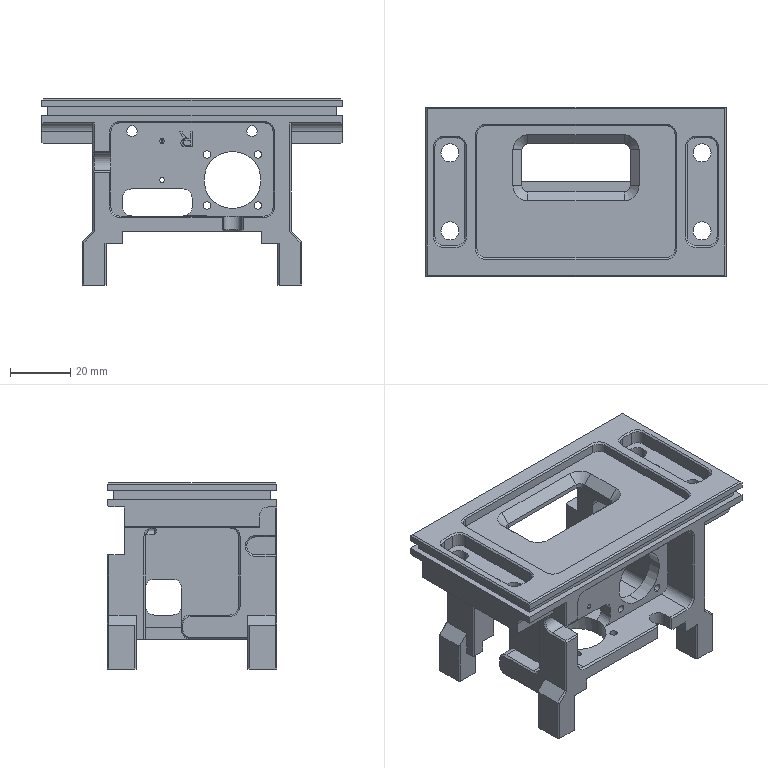NC program | Mastercam | posted with a generic post | part box 100 x 56.5 x 62 mm
Lines 34 to 1359 of 47040:
N260 T13 M6
N270 G0 G90 G17 G54 X-64.057 Y-49.411 A0. S5500 M3
N280 G43 H13 Z20. M8
N290 Z1.
N300 G1 Z-28.25 F600.
N310 X-64.59 Y-48.087 Z-28.374 F3000.
N320 G3 X-65.384 Y-46.884 Z-28.5 I-3.34 J-1.343
N330 G1 X-65.592 Y-46.603
N340 X-66.057 Y-45.951
N350 X-66.342 Y-45.52
N360 X-66.635 Y-45.037
N370 X-66.924 Y-44.51
N380 X-67.198 Y-43.943
N390 X-67.451 Y-43.341
N400 X-67.673 Y-42.718
N410 X-67.849 Y-42.127
N420 X-67.986 Y-41.577
N430 X-68.092 Y-41.064
N440 X-68.174 Y-40.586
N450 X-68.238 Y-40.138
N460 X-68.326 Y-39.34
N470 X-68.382 Y-38.609
N480 X-68.418 Y-37.931
N490 X-68.441 Y-37.291
N500 X-68.456 Y-36.678
N510 X-68.465 Y-36.084
N520 X-68.471 Y-35.505
N530 X-68.474 Y-34.935
N540 X-68.475 Y-34.371
N550 X-68.476 Y-33.813
N560 X-68.475 Y-33.258
N570 X-68.474 Y-32.705
N580 X-68.473 Y-32.153
N590 X-68.472 Y-31.603
N600 X-68.471 Y-31.052
N610 X-68.469 Y-30.502
N620 X-68.467 Y-29.953
N630 X-68.466 Y-29.403
N640 X-68.464 Y-28.853
N650 X-68.463 Y-28.304
N660 X-68.461 Y-27.754
N670 X-68.459 Y-27.205
N680 X-68.458 Y-26.655
N690 X-68.456 Y-26.105
N700 X-68.455 Y-25.556
N710 X-68.453 Y-25.006
N720 X-68.451 Y-24.456
N730 X-68.45 Y-23.906
N740 X-68.448 Y-23.357
N750 X-68.446 Y-22.807
N760 X-68.445 Y-22.257
N770 X-68.443 Y-21.707
N780 X-68.442 Y-21.157
N790 X-68.44 Y-20.607
N800 X-68.438 Y-20.057
N810 X-68.437 Y-19.507
N820 X-68.435 Y-18.957
N830 X-68.433 Y-18.407
N840 X-68.432 Y-17.857
N850 X-68.43 Y-17.307
N860 X-68.429 Y-16.757
N870 X-68.427 Y-16.207
N880 X-68.425 Y-15.656
N890 X-68.424 Y-15.106
N900 X-68.422 Y-14.556
N910 X-68.42 Y-14.006
N920 X-68.419 Y-13.456
N930 X-68.417 Y-12.905
N940 X-68.416 Y-12.355
N950 X-68.414 Y-11.805
N960 X-68.412 Y-11.254
N970 X-68.411 Y-10.704
N980 X-68.409 Y-10.153
N990 X-68.407 Y-9.603
N1000 X-68.406 Y-9.052
N1010 X-68.404 Y-8.502
N1020 X-68.403 Y-7.951
N1030 X-68.401 Y-7.401
N1040 X-68.399 Y-6.85
N1050 X-68.398 Y-6.3
N1060 X-68.396 Y-5.749
N1070 X-68.394 Y-5.199
N1080 X-68.393 Y-4.648
N1090 X-68.391 Y-4.097
N1100 X-68.39 Y-3.547
N1110 X-68.388 Y-2.996
N1120 X-68.386 Y-2.445
N1130 X-68.385 Y-1.895
N1140 X-68.383 Y-1.344
N1150 X-68.381 Y-.793
N1160 X-68.38 Y-.242
N1170 X-68.378 Y.309
N1180 X-68.377 Y.859
N1190 X-68.375 Y1.41
N1200 X-68.373 Y1.961
N1210 X-68.372 Y2.512
N1220 X-68.37 Y3.063
N1230 X-68.368 Y3.614
N1240 X-68.367 Y4.165
N1250 X-68.365 Y4.716
N1260 X-68.363 Y5.267
N1270 X-68.362 Y5.818
N1280 X-68.36 Y6.369
N1290 X-68.359 Y6.92
N1300 X-68.357 Y7.471
N1310 X-68.355 Y8.022
N1320 X-68.354 Y8.573
N1330 X-68.352 Y9.124
N1340 X-68.35 Y9.675
N1350 X-68.349 Y10.226
N1360 X-68.347 Y10.778
N1370 X-68.346 Y11.329
N1380 X-68.344 Y11.88
N1390 X-68.342 Y12.431
N1400 X-68.341 Y12.982
N1410 X-68.339 Y13.534
N1420 X-68.337 Y14.085
N1430 X-68.336 Y14.636
N1440 X-68.334 Y15.187
N1450 X-68.333 Y15.739
N1460 X-68.331 Y16.29
N1470 X-68.329 Y16.841
N1480 X-68.328 Y17.393
N1490 X-68.326 Y17.944
N1500 X-68.324 Y18.495
N1510 X-68.323 Y19.047
N1520 X-68.321 Y19.598
N1530 X-68.319 Y20.149
N1540 X-68.318 Y20.701
N1550 X-68.316 Y21.252
N1560 X-68.315 Y21.804
N1570 X-68.313 Y22.355
N1580 X-68.311 Y22.907
N1590 X-68.31 Y23.458
N1600 X-68.308 Y24.01
N1610 X-68.306 Y24.561
N1620 X-68.305 Y25.113
N1630 X-68.303 Y25.664
N1640 X-68.302 Y26.216
N1650 X-68.3 Y26.767
N1660 X-68.298 Y27.319
N1670 X-68.297 Y27.871
N1680 X-68.295 Y28.422
N1690 X-68.293 Y28.974
N1700 X-68.292 Y29.525
N1710 X-68.29 Y30.077
N1720 X-68.288 Y30.629
N1730 X-68.287 Y31.18
N1740 X-68.285 Y31.732
N1750 X-68.284 Y32.284
N1760 X-68.282 Y32.836
N1770 X-68.28 Y33.387
N1780 X-68.279 Y33.939
N1790 X-68.277 Y34.491
N1800 X-68.275 Y35.043
N1810 X-68.274 Y35.594
N1820 X-68.272 Y36.146
N1830 X-68.27 Y36.705
N1840 X-68.26 Y37.428
N1850 X-68.241 Y37.868
N1860 X-68.208 Y38.345
N1870 X-68.157 Y38.854
N1880 X-68.082 Y39.387
N1890 X-67.981 Y39.94
N1900 X-67.852 Y40.507
N1910 X-67.69 Y41.084
N1920 X-67.495 Y41.665
N1930 X-67.265 Y42.248
N1940 X-66.998 Y42.826
N1950 X-66.694 Y43.397
N1960 X-66.352 Y43.955
N1970 X-65.973 Y44.498
N1980 X-65.558 Y45.022
N1990 X-65.107 Y45.522
N2000 X-64.621 Y45.996
N2010 X-64.106 Y46.436
N2020 X-63.582 Y46.831
N2030 X-63.056 Y47.181
N2040 X-62.533 Y47.489
N2050 X-62.016 Y47.76
N2060 X-61.509 Y47.998
N2070 X-61.014 Y48.205
N2080 X-60.531 Y48.386
N2090 X-60.061 Y48.543
N2100 X-59.605 Y48.681
N2110 X-59.163 Y48.8
N2120 X-58.733 Y48.904
N2130 X-57.927 Y49.071
N2140 X-57.16 Y49.201
N2150 X-56.428 Y49.301
N2160 X-55.726 Y49.378
N2170 X-55.05 Y49.439
N2180 X-54.397 Y49.486
N2190 X-53.761 Y49.523
N2200 X-53.141 Y49.552
N2210 X-52.533 Y49.574
N2220 X-51.936 Y49.592
N2230 X-51.347 Y49.606
N2240 X-50.765 Y49.616
N2250 X-50.189 Y49.624
N2260 X-49.617 Y49.63
N2270 X-49.049 Y49.635
N2280 X-48.485 Y49.638
N2290 X-47.923 Y49.64
N2300 X-47.361 Y49.642
N2310 X-46.801 Y49.643
N2320 X-46.241 Y49.645
N2330 X-45.681 Y49.646
N2340 X-45.123
N2350 X-44.564 Y49.647
N2360 X-44.006 Y49.648
N2370 X-43.448
N2380 X-42.89
N2390 X-42.332 Y49.649
N2400 X-41.775
N2410 X-41.218
N2420 X-40.66
N2430 X-40.103
N2440 X-39.546
N2450 X-38.989 Y49.65
N2460 X-38.432
N2470 X-37.874
N2480 X-37.317
N2490 X-36.76
N2500 X-36.203
N2510 X-35.646
N2520 X-35.089
N2530 X-34.532
N2540 X-33.976
N2550 X-33.419
N2560 X-32.862
N2570 X-32.305
N2580 X-31.748
N2590 X-31.191
N2600 X-30.634
N2610 X-30.077
N2620 X-29.52
N2630 X-28.963
N2640 X-28.406
N2650 X-27.849
N2660 X-27.292
N2670 X-26.735
N2680 X-26.179
N2690 X-25.622
N2700 X-25.065
N2710 X-24.508
N2720 X-23.951
N2730 X-23.394
N2740 X-22.837
N2750 X-22.28
N2760 X-21.723
N2770 X-21.166
N2780 X-20.609
N2790 X-20.053
N2800 X-19.496
N2810 X-18.939
N2820 X-18.382
N2830 X-17.825
N2840 X-17.268
N2850 X-16.711
N2860 X-16.154
N2870 X-15.597
N2880 X-15.04
N2890 X-14.483
N2900 X-13.927
N2910 X-13.37
N2920 X-12.813
N2930 X-12.256
N2940 X-11.699
N2950 X-11.142
N2960 X-10.585
N2970 X-10.028
N2980 X-9.471
N2990 X-8.914
N3000 X-8.357
N3010 X-7.801
N3020 X-7.244
N3030 X-6.687
N3040 X-6.13
N3050 X-5.573
N3060 X-5.016
N3070 X-4.459
N3080 X-3.902
N3090 X-3.345
N3100 X-2.788
N3110 X-2.231
N3120 X-1.675
N3130 X-1.118
N3140 X-.561
N3150 X-.004
N3160 X.553
N3170 X1.11
N3180 X1.667
N3190 X2.224
N3200 X2.781
N3210 X3.338
N3220 X3.895
N3230 X4.452
N3240 X5.008
N3250 X5.565
N3260 X6.122
N3270 X6.679
N3280 X7.236
N3290 X7.793
N3300 X8.35
N3310 X8.907
N3320 X9.464
N3330 X10.021
N3340 X10.578
N3350 X11.134
N3360 X11.691
N3370 X12.248
N3380 X12.805
N3390 X13.362
N3400 X13.919
N3410 X14.476
N3420 X15.033
N3430 X15.59
N3440 X16.147
N3450 X16.704
N3460 X17.26
N3470 X17.817
N3480 X18.374
N3490 X18.931
N3500 X19.488
N3510 X20.045
N3520 X20.602
N3530 X21.159
N3540 X21.716
N3550 X22.273
N3560 X22.83
N3570 X23.386
N3580 X23.943
N3590 X24.5
N3600 X25.057
N3610 X25.614
N3620 X26.171
N3630 X26.728
N3640 X27.285
N3650 X27.842
N3660 X28.399
N3670 X28.956
N3680 X29.512
N3690 X30.069
N3700 X30.626
N3710 X31.183
N3720 X31.74
N3730 X32.297
N3740 X32.854
N3750 X33.411
N3760 X33.968
N3770 X34.525
N3780 X35.082
N3790 X35.638
N3800 X36.195
N3810 X36.752
N3820 X37.309
N3830 X37.866
N3840 X38.423
N3850 X38.98
N3860 X39.537
N3870 X40.094
N3880 X40.651
N3890 X41.208
N3900 X41.765
N3910 X42.321
N3920 X42.878
N3930 X43.435
N3940 X43.992
N3950 X44.549
N3960 X45.106
N3970 X45.663
N3980 X46.22
N3990 X46.777
N4000 X47.334
N4010 X47.891
N4020 X48.447
N4030 X49.004
N4040 X49.561
N4050 X50.118
N4060 X50.675
N4070 X51.232
N4080 X51.789
N4090 X52.346
N4100 X52.903
N4110 X53.46
N4120 X54.017
N4130 X54.573
N4140 X55.19 Y49.649
N4150 X55.986 Y49.629
N4160 X56.447 Y49.602
N4170 X56.938 Y49.559
N4180 X57.453 Y49.495
N4190 X57.988 Y49.409
N4200 X58.538 Y49.296
N4210 X59.1 Y49.154
N4220 X59.667 Y48.981
N4230 X60.238 Y48.776
N4240 X60.807 Y48.536
N4250 X61.372 Y48.26
N4260 X61.927 Y47.949
N4270 X62.47 Y47.602
N4280 X62.996 Y47.218
N4290 X63.503 Y46.8
N4300 X63.986 Y46.346
N4310 X64.439 Y45.864
N4320 X64.85 Y45.368
N4330 X65.221 Y44.865
N4340 X65.553 Y44.36
N4350 X65.85 Y43.856
N4360 X66.113 Y43.356
N4370 X66.347 Y42.864
N4380 X66.554 Y42.38
N4390 X66.737 Y41.907
N4400 X66.898 Y41.444
N4410 X67.04 Y40.992
N4420 X67.165 Y40.552
N4430 X67.276 Y40.123
N4440 X67.456 Y39.314
N4450 X67.597 Y38.541
N4460 X67.708 Y37.8
N4470 X67.796 Y37.089
N4480 X67.866 Y36.403
N4490 X67.921 Y35.738
N4500 X67.965 Y35.092
N4510 X68. Y34.461
N4520 X68.029 Y33.843
N4530 X68.052 Y33.236
N4540 X68.07 Y32.638
N4550 X68.085 Y32.047
N4560 X68.097 Y31.462
N4570 X68.107 Y30.882
N4580 X68.115 Y30.306
N4590 X68.121 Y29.734
N4600 X68.127 Y29.164
N4610 X68.131 Y28.597
N4620 X68.134 Y28.031
N4630 X68.137 Y27.467
N4640 X68.14 Y26.905
N4650 X68.141 Y26.343
N4660 X68.143 Y25.783
N4670 X68.144 Y25.223
N4680 X68.145 Y24.663
N4690 X68.146 Y24.104
N4700 X68.147 Y23.545
N4710 Y22.987
N4720 X68.148 Y22.429
N4730 Y21.871
N4740 X68.149 Y21.314
N4750 Y20.756
N4760 Y20.199
N4770 Y19.641
N4780 Y19.084
N4790 Y18.527
N4800 X68.15 Y17.97
N4810 Y17.413
N4820 Y16.855
N4830 Y16.298
N4840 Y15.741
N4850 Y15.184
N4860 Y14.627
N4870 Y14.07
N4880 Y13.513
N4890 Y12.956
N4900 Y12.4
N4910 Y11.843
N4920 Y11.286
N4930 Y10.729
N4940 Y10.172
N4950 Y9.615
N4960 Y9.058
N4970 Y8.501
N4980 Y7.944
N4990 Y7.387
N5000 Y6.83
N5010 Y6.273
N5020 Y5.716
N5030 Y5.16
N5040 Y4.603
N5050 Y4.046
N5060 Y3.489
N5070 Y2.932
N5080 Y2.375
N5090 Y1.818
N5100 Y1.261
N5110 Y.704
N5120 Y.147
N5130 Y-.41
N5140 Y-.967
N5150 Y-1.523
N5160 Y-2.08
N5170 Y-2.637
N5180 Y-3.194
N5190 Y-3.751
N5200 Y-4.308
N5210 Y-4.865
N5220 Y-5.422
N5230 Y-5.979
N5240 Y-6.536
N5250 Y-7.093
N5260 Y-7.649
N5270 Y-8.206
N5280 Y-8.763
N5290 Y-9.32
N5300 Y-9.877
N5310 Y-10.434
N5320 Y-10.991
N5330 Y-11.548
N5340 Y-12.105
N5350 Y-12.662
N5360 Y-13.219
N5370 Y-13.775
N5380 Y-14.332
N5390 Y-14.889
N5400 Y-15.446
N5410 Y-16.003
N5420 Y-16.56
N5430 Y-17.117
N5440 Y-17.674
N5450 Y-18.231
N5460 Y-18.788
N5470 Y-19.345
N5480 Y-19.901
N5490 Y-20.458
N5500 Y-21.015
N5510 Y-21.572
N5520 Y-22.129
N5530 Y-22.686
N5540 Y-23.243
N5550 Y-23.8
N5560 Y-24.357
N5570 Y-24.914
N5580 Y-25.471
N5590 Y-26.027
N5600 Y-26.584
N5610 Y-27.141
N5620 Y-27.698
N5630 Y-28.255
N5640 Y-28.812
N5650 Y-29.369
N5660 Y-29.926
N5670 Y-30.483
N5680 Y-31.04
N5690 Y-31.597
N5700 Y-32.153
N5710 Y-32.71
N5720 Y-33.267
N5730 Y-33.824
N5740 Y-34.381
N5750 Y-34.938
N5760 Y-35.495
N5770 Y-36.052
N5780 X68.149 Y-36.662
N5790 X68.13 Y-37.452
N5800 X68.104 Y-37.911
N5810 X68.062 Y-38.399
N5820 X68.001 Y-38.913
N5830 X67.916 Y-39.447
N5840 X67.805 Y-39.996
N5850 X67.666 Y-40.557
N5860 X67.496 Y-41.124
N5870 X67.292 Y-41.695
N5880 X67.055 Y-42.264
N5890 X66.782 Y-42.829
N5900 X66.474 Y-43.385
N5910 X66.129 Y-43.929
N5920 X65.749 Y-44.457
N5930 X65.333 Y-44.965
N5940 X64.882 Y-45.45
N5950 X64.401 Y-45.906
N5960 X63.906 Y-46.32
N5970 X63.403 Y-46.694
N5980 X62.898 Y-47.029
N5990 X62.394 Y-47.328
N6000 X61.894 Y-47.595
N6010 X61.401 Y-47.831
N6020 X60.917 Y-48.039
N6030 X60.442 Y-48.224
N6040 X59.979 Y-48.386
N6050 X59.526 Y-48.53
N6060 X59.085 Y-48.656
N6070 X58.655 Y-48.768
N6080 X57.844 Y-48.95
N6090 X57.07 Y-49.092
N6100 X56.328 Y-49.205
N6110 X55.616 Y-49.293
N6120 X54.929 Y-49.363
N6130 X54.264 Y-49.419
N6140 X53.617 Y-49.464
N6150 X52.985 Y-49.499
N6160 X52.367 Y-49.528
N6170 X51.759 Y-49.551
N6180 X51.161 Y-49.569
N6190 X50.569 Y-49.584
N6200 X49.984 Y-49.597
N6210 X49.404 Y-49.606
N6220 X48.828 Y-49.614
N6230 X48.256 Y-49.621
N6240 X47.686 Y-49.626
N6250 X47.119 Y-49.631
N6260 X46.553 Y-49.634
N6270 X45.989 Y-49.637
N6280 X45.427 Y-49.639
N6290 X44.865 Y-49.641
N6300 X44.304 Y-49.643
N6310 X43.744 Y-49.644
N6320 X43.185 Y-49.645
N6330 X42.626 Y-49.646
N6340 X42.067 Y-49.647
N6350 X41.509
N6360 X40.951 Y-49.648
N6370 X40.393
N6380 X39.835 Y-49.649
N6390 X39.278
N6400 X38.72
N6410 X38.163
N6420 X37.606
N6430 X37.048
N6440 X36.491 Y-49.65
N6450 X35.934
N6460 X35.377
N6470 X34.82
N6480 X34.263
N6490 X33.706
N6500 X33.149
N6510 X32.592
N6520 X32.035
N6530 X31.478
N6540 X30.921
N6550 X30.364
N6560 X29.807
N6570 X29.25
N6580 X28.693
N6590 X28.136
N6600 X27.58
N6610 X27.023
N6620 X26.466
N6630 X25.909
N6640 X25.352
N6650 X24.795
N6660 X24.238
N6670 X23.681
N6680 X23.124
N6690 X22.567
N6700 X22.01
N6710 X21.453
N6720 X20.897
N6730 X20.34
N6740 X19.783
N6750 X19.226
N6760 X18.669
N6770 X18.112
N6780 X17.555
N6790 X16.998
N6800 X16.441
N6810 X15.884
N6820 X15.327
N6830 X14.771
N6840 X14.214
N6850 X13.657
N6860 X13.1
N6870 X12.543
N6880 X11.986
N6890 X11.429
N6900 X10.872
N6910 X10.315
N6920 X9.758
N6930 X9.201
N6940 X8.645
N6950 X8.088
N6960 X7.531
N6970 X6.974
N6980 X6.417
N6990 X5.86
N7000 X5.303
N7010 X4.746
N7020 X4.189
N7030 X3.632
N7040 X3.075
N7050 X2.519
N7060 X1.962
N7070 X1.405
N7080 X.848
N7090 X.291
N7100 X-.266
N7110 X-.823
N7120 X-1.38
N7130 X-1.937
N7140 X-2.494
N7150 X-3.051
N7160 X-3.608
N7170 X-4.164
N7180 X-4.721
N7190 X-5.278
N7200 X-5.835
N7210 X-6.392
N7220 X-6.949
N7230 X-7.506
N7240 X-8.063
N7250 X-8.62
N7260 X-9.177
N7270 X-9.734
N7280 X-10.29
N7290 X-10.847
N7300 X-11.404
N7310 X-11.961
N7320 X-12.518
N7330 X-13.075
N7340 X-13.632
N7350 X-14.189
N7360 X-14.746
N7370 X-15.303
N7380 X-15.86
N7390 X-16.416
N7400 X-16.973
N7410 X-17.53
N7420 X-18.087
N7430 X-18.644
N7440 X-19.201
N7450 X-19.758
N7460 X-20.315
N7470 X-20.872
N7480 X-21.429
N7490 X-21.986
N7500 X-22.542
N7510 X-23.099
N7520 X-23.656
N7530 X-24.213
N7540 X-24.77
N7550 X-25.327
N7560 X-25.884
N7570 X-26.441
N7580 X-26.998
N7590 X-27.555
N7600 X-28.112
N7610 X-28.668
N7620 X-29.225
N7630 X-29.782
N7640 X-30.339
N7650 X-30.896
N7660 X-31.453
N7670 X-32.01
N7680 X-32.567
N7690 X-33.124
N7700 X-33.681
N7710 X-34.238
N7720 X-34.794
N7730 X-35.351
N7740 X-35.908
N7750 X-36.465
N7760 X-37.022
N7770 X-37.579
N7780 X-38.136
N7790 X-38.693
N7800 X-39.25
N7810 X-39.807
N7820 X-40.364
N7830 X-40.92
N7840 X-41.477
N7850 X-42.034
N7860 X-42.591
N7870 X-43.148
N7880 X-43.705
N7890 X-44.262
N7900 X-44.819
N7910 X-45.376
N7920 X-45.933
N7930 X-46.49
N7940 X-47.047
N7950 X-47.603
N7960 X-48.16
N7970 X-48.717
N7980 X-49.274
N7990 X-49.831
N8000 X-50.388
N8010 X-50.945
N8020 X-51.502
N8030 X-52.059
N8040 X-52.616
N8050 X-53.173
N8060 X-53.729
N8070 X-54.286
N8080 X-54.849
N8090 X-55.557 Y-49.643
N8100 X-55.982 Y-49.629
N8110 X-56.443 Y-49.602
N8120 X-56.933 Y-49.559
N8130 X-57.449 Y-49.496
N8140 X-57.984 Y-49.409
N8150 X-58.623 Y-49.273
N8160 X-59.257 Y-49.095
N8170 X-59.874 Y-48.881
N8180 X-60.475 Y-48.629
N8190 X-61.062 Y-48.34
N8200 X-61.631 Y-48.016
N8210 X-62.177 Y-47.658
N8220 X-62.698 Y-47.27
N8230 X-63.189 Y-46.855
N8240 X-63.65 Y-46.419
N8250 X-64.08 Y-45.962
N8260 X-64.472 Y-45.497
N8270 X-64.835 Y-45.02
N8280 X-65.164 Y-44.54
N8290 X-65.464 Y-44.055
N8300 X-65.734 Y-43.573
N8310 X-65.979 Y-43.092
N8320 X-66.197 Y-42.618
N8330 X-66.393 Y-42.148
N8340 X-66.567 Y-41.688
N8350 X-66.723 Y-41.235
N8360 X-66.861 Y-40.792
N8370 X-66.985 Y-40.358
N8380 X-67.094 Y-39.934
N8390 X-67.274 Y-39.13
N8400 X-67.416 Y-38.359
N8410 X-67.529 Y-37.618
N8420 X-67.618 Y-36.904
N8430 X-67.688 Y-36.215
N8440 X-67.744 Y-35.547
N8450 X-67.788 Y-34.898
N8460 X-67.823 Y-34.264
N8470 X-67.851 Y-33.644
N8480 X-67.873 Y-33.034
N8490 X-67.891 Y-32.434
N8500 X-67.905 Y-31.842
N8510 X-67.916 Y-31.255
N8520 X-67.924 Y-30.674
N8530 X-67.931 Y-30.098
N8540 X-67.936 Y-29.525
N8550 X-67.94 Y-28.954
N8560 X-67.943 Y-28.387
N8570 X-67.945 Y-27.821
N8580 X-67.946 Y-27.256
N8590 X-67.947 Y-26.694
N8600 Y-26.132
N8610 Y-25.571
N8620 Y-25.011
N8630 X-67.946 Y-24.451
N8640 Y-23.892
N8650 X-67.945 Y-23.333
N8660 X-67.944 Y-22.775
N8670 X-67.943 Y-22.217
N8680 X-67.941 Y-21.659
N8690 X-67.94 Y-21.101
N8700 X-67.939 Y-20.544
N8710 X-67.937 Y-19.986
N8720 X-67.936 Y-19.429
N8730 X-67.934 Y-18.871
N8740 X-67.933 Y-18.314
N8750 X-67.931 Y-17.757
N8760 X-67.93 Y-17.2
N8770 X-67.928 Y-16.643
N8780 X-67.926 Y-16.086
N8790 X-67.925 Y-15.529
N8800 X-67.923 Y-14.972
N8810 X-67.922 Y-14.415
N8820 X-67.92 Y-13.858
N8830 X-67.918 Y-13.301
N8840 X-67.917 Y-12.744
N8850 X-67.915 Y-12.187
N8860 X-67.913 Y-11.63
N8870 X-67.912 Y-11.073
N8880 X-67.91 Y-10.516
N8890 X-67.908 Y-9.959
N8900 X-67.907 Y-9.402
N8910 X-67.905 Y-8.845
N8920 X-67.904 Y-8.288
N8930 X-67.902 Y-7.732
N8940 X-67.9 Y-7.175
N8950 X-67.899 Y-6.618
N8960 X-67.897 Y-6.061
N8970 X-67.895 Y-5.504
N8980 X-67.894 Y-4.947
N8990 X-67.892 Y-4.39
N9000 X-67.89 Y-3.833
N9010 X-67.889 Y-3.276
N9020 X-67.887 Y-2.719
N9030 X-67.885 Y-2.162
N9040 X-67.884 Y-1.606
N9050 X-67.882 Y-1.049
N9060 X-67.88 Y-.492
N9070 X-67.879 Y.065
N9080 X-67.877 Y.622
N9090 X-67.876 Y1.179
N9100 X-67.874 Y1.736
N9110 X-67.872 Y2.293
N9120 X-67.871 Y2.85
N9130 X-67.869 Y3.407
N9140 X-67.867 Y3.964
N9150 X-67.866 Y4.52
N9160 X-67.864 Y5.077
N9170 X-67.862 Y5.634
N9180 X-67.861 Y6.191
N9190 X-67.859 Y6.748
N9200 X-67.857 Y7.305
N9210 X-67.856 Y7.862
N9220 X-67.854 Y8.419
N9230 X-67.853 Y8.976
N9240 X-67.851 Y9.533
N9250 X-67.849 Y10.09
N9260 X-67.848 Y10.646
N9270 X-67.846 Y11.203
N9280 X-67.844 Y11.76
N9290 X-67.843 Y12.317
N9300 X-67.841 Y12.874
N9310 X-67.839 Y13.431
N9320 X-67.838 Y13.988
N9330 X-67.836 Y14.545
N9340 X-67.834 Y15.102
N9350 X-67.833 Y15.659
N9360 X-67.831 Y16.216
N9370 X-67.829 Y16.772
N9380 X-67.828 Y17.329
N9390 X-67.826 Y17.886
N9400 X-67.825 Y18.443
N9410 X-67.823 Y19.
N9420 X-67.821 Y19.557
N9430 X-67.82 Y20.114
N9440 X-67.818 Y20.671
N9450 X-67.816 Y21.228
N9460 X-67.815 Y21.785
N9470 X-67.813 Y22.342
N9480 X-67.811 Y22.898
N9490 X-67.81 Y23.455
N9500 X-67.808 Y24.012
N9510 X-67.806 Y24.569
N9520 X-67.805 Y25.126
N9530 X-67.803 Y25.683
N9540 X-67.801 Y26.24
N9550 X-67.8 Y26.797
N9560 X-67.798 Y27.354
N9570 X-67.797 Y27.911
N9580 X-67.795 Y28.468
N9590 X-67.793 Y29.024
N9600 X-67.792 Y29.581
N9610 X-67.79 Y30.138
N9620 X-67.788 Y30.695
N9630 X-67.787 Y31.252
N9640 X-67.785 Y31.809
N9650 X-67.783 Y32.366
N9660 X-67.782 Y32.923
N9670 X-67.78 Y33.48
N9680 X-67.778 Y34.041
N9690 X-67.775 Y34.621
N9700 X-67.767 Y35.267
N9710 X-67.743 Y36.003
N9720 X-67.688 Y36.834
N9730 X-67.64 Y37.299
N9740 X-67.575 Y37.788
N9750 X-67.487 Y38.306
N9760 X-67.375 Y38.842
N9770 X-67.232 Y39.4
N9780 X-67.056 Y39.972
N9790 X-66.845 Y40.549
N9800 X-66.6 Y41.121
N9810 X-66.322 Y41.683
N9820 X-66.014 Y42.227
N9830 X-65.677 Y42.751
N9840 X-65.316 Y43.251
N9850 X-64.933 Y43.727
N9860 X-64.53 Y44.177
N9870 X-64.109 Y44.6
N9880 X-63.676 Y44.996
N9890 X-63.238 Y45.361
N9900 X-62.79 Y45.701
N9910 X-62.339 Y46.013
N9920 X-61.884 Y46.302
N9930 X-61.431 Y46.567
N9940 X-60.978 Y46.809
N9950 X-60.528 Y47.03
N9960 X-60.081 Y47.231
N9970 X-59.64 Y47.414
N9980 X-59.204 Y47.581
N9990 X-58.775 Y47.732
N100 X-58.352 Y47.868
N110 X-57.936 Y47.992
N120 X-57.14 Y48.201
N130 X-56.369 Y48.373
N140 X-55.622 Y48.514
N150 X-54.899 Y48.63
N160 X-54.196 Y48.724
N170 X-53.513 Y48.801
N180 X-52.848 Y48.864
N190 X-52.197 Y48.916
N200 X-51.56 Y48.958
N210 X-50.936 Y48.992
N220 X-50.322 Y49.02
N230 X-49.717 Y49.043
N240 X-49.121 Y49.062
N250 X-48.531 Y49.078
N260 X-47.946 Y49.09
N270 X-47.367 Y49.101
N280 X-46.791 Y49.109
N290 X-46.218 Y49.116
N300 X-45.648 Y49.122
N310 X-45.08 Y49.127
N320 X-44.514 Y49.131
N330 X-43.95 Y49.134
N340 X-43.386 Y49.137
N350 X-42.824 Y49.139
N360 X-42.263 Y49.141
N370 X-41.703 Y49.143
N380 X-41.143 Y49.144
N390 X-40.584 Y49.145
N400 X-40.025 Y49.146
N410 X-39.466 Y49.147
N420 X-38.908
N430 X-38.35 Y49.148
N440 X-37.792
N450 X-37.234
N460 X-36.677 Y49.149
N470 X-36.119
N480 X-35.562
N490 X-35.005
N500 X-34.447
N510 X-33.89
N520 X-33.333 Y49.15
N530 X-32.776
N540 X-32.219
N550 X-31.662
N560 X-31.105
N570 X-30.548
N580 X-29.991
N590 X-29.434
N600 X-28.877
N610 X-28.32
N620 X-27.763
N630 X-27.206
N640 X-26.649
N650 X-26.092
N660 X-25.535
N670 X-24.978
N680 X-24.421
N690 X-23.864
N700 X-23.308
N710 X-22.751
N720 X-22.194
N730 X-21.637
N740 X-21.08
N750 X-20.523
N760 X-19.966
N770 X-19.409
N780 X-18.852
N790 X-18.295
N800 X-17.738
N810 X-17.181
N820 X-16.625
N830 X-16.068
N840 X-15.511
N850 X-14.954
N860 X-14.397
N870 X-13.84
N880 X-13.283
N890 X-12.726
N900 X-12.169
N910 X-11.612
N920 X-11.055
N930 X-10.499
N940 X-9.942
N950 X-9.385
N960 X-8.828
N970 X-8.271
N980 X-7.714
N990 X-7.157
N1000 X-6.6
N1010 X-6.043
N1020 X-5.486
N1030 X-4.929
N1040 X-4.373
N1050 X-3.816
N1060 X-3.259
N1070 X-2.702
N1080 X-2.145
N1090 X-1.588
N1100 X-1.031
N1110 X-.474
N1120 X.083
N1130 X.64
N1140 X1.197
N1150 X1.753
N1160 X2.31
N1170 X2.867
N1180 X3.424
N1190 X3.981
N1200 X4.538
N1210 X5.095
N1220 X5.652
N1230 X6.209
N1240 X6.766
N1250 X7.323
N1260 X7.88
N1270 X8.436
N1280 X8.993
N1290 X9.55
N1300 X10.107
N1310 X10.664
N1320 X11.221
N1330 X11.778
N1340 X12.335
N1350 X12.892
N1360 X13.449
N1370 X14.006
N1380 X14.562
N1390 X15.119
N1400 X15.676
N1410 X16.233
N1420 X16.79
N1430 X17.347
N1440 X17.904
N1450 X18.461
N1460 X19.018
N1470 X19.575
N1480 X20.132
N1490 X20.688
N1500 X21.245
N1510 X21.802
N1520 X22.359
N1530 X22.916
N1540 X23.473
N1550 X24.03
N1560 X24.587
N1570 X25.144
N1580 X25.701
N1590 X26.258
N1600 X26.814
N1610 X27.371
N1620 X27.928
N1630 X28.485
N1640 X29.042
N1650 X29.599
N1660 X30.156
N1670 X30.713
N1680 X31.27
N1690 X31.827
N1700 X32.384
N1710 X32.94
N1720 X33.497
N1730 X34.054
N1740 X34.611
N1750 X35.168
N1760 X35.725
N1770 X36.282
N1780 X36.839
N1790 X37.396
N1800 X37.953
N1810 X38.51
N1820 X39.066
N1830 X39.623
N1840 X40.18
N1850 X40.737
N1860 X41.294
N1870 X41.851
N1880 X42.408
N1890 X42.965
N1900 X43.522
N1910 X44.079
N1920 X44.636
N1930 X45.193
N1940 X45.749
N1950 X46.306
N1960 X46.863
N1970 X47.42
N1980 X47.977
N1990 X48.534
N2000 X49.091
N2010 X49.648
N2020 X50.205
N2030 X50.762
N2040 X51.319
N2050 X51.876
N2060 X52.443
N2070 X53.037 Y49.147
N2080 X53.702 Y49.138
N2090 X54.455 Y49.111
N2100 X54.874 Y49.084
N2110 X55.319 Y49.046
N2120 X55.793 Y48.993
N2130 X56.291 Y48.92
N2140 X56.815 Y48.825
N2150 X57.361 Y48.702
N2160 X57.925 Y48.548
N2170 X58.501 Y48.36
N2180 X59.073 Y48.139
N2190 X59.638 Y47.885
N2200 X60.19 Y47.6
N2210 X60.723 Y47.286
N2220 X61.234 Y46.947
N2230 X61.723 Y46.585
N2240 X62.187 Y46.203
N2250 X62.625 Y45.802
N2260 X63.039 Y45.386
N2270 X63.427 Y44.957
N2280 X63.784 Y44.525
N2290 X64.118 Y44.081
N2300 X64.426 Y43.638
N2310 X64.711 Y43.188
N2320 X64.972 Y42.742
N2330 X65.214 Y42.293
N2340 X65.433 Y41.85
N2350 X65.635 Y41.408
N2360 X65.818 Y40.972
N2370 X65.986 Y40.54
N2380 X66.138 Y40.115
N2390 X66.277 Y39.695
N2400 X66.403 Y39.282
N2410 X66.618 Y38.491
N2420 X66.795 Y37.723
N2430 X66.942 Y36.979
N2440 X67.063 Y36.256
N2450 X67.163 Y35.554
N2460 X67.246 Y34.87
N2470 X67.314 Y34.203
N2480 X67.371 Y33.552
N2490 X67.418 Y32.913
N2500 X67.457 Y32.287
N2510 X67.489 Y31.67
N2520 X67.516 Y31.063
N2530 X67.538 Y30.463
N2540 X67.557 Y29.869
N2550 X67.572 Y29.281
N2560 X67.585 Y28.698
N2570 X67.596 Y28.119
N2580 X67.605 Y27.543
N2590 X67.613 Y26.971
N2600 X67.619 Y26.401
N2610 X67.624 Y25.833
N2620 X67.628 Y25.266
N2630 X67.632 Y24.702
N2640 X67.635 Y24.138
N2650 X67.637 Y23.576
N2660 X67.64 Y23.014
N2670 X67.641 Y22.453
N2680 X67.643 Y21.893
N2690 X67.644 Y21.334
N2700 X67.645 Y20.775
N2710 X67.646 Y20.216
N2720 X67.647 Y19.657
N2730 Y19.099
N2740 X67.648 Y18.541
N2750 Y17.983
N2760 Y17.426
N2770 X67.649 Y16.868
N2780 Y16.311
N2790 Y15.753
N2800 Y15.196
N2810 Y14.639
N2820 Y14.082
N2830 X67.65 Y13.524
N2840 Y12.967
N2850 Y12.41
N2860 Y11.853
N2870 Y11.296
N2880 Y10.739
N2890 Y10.182
N2900 Y9.625
N2910 Y9.068
N2920 Y8.511
N2930 Y7.954
N2940 Y7.397
N2950 Y6.84
N2960 Y6.283
N2970 Y5.727
N2980 Y5.17
N2990 Y4.613
N3000 Y4.056
N3010 Y3.499
N3020 Y2.942
N3030 Y2.385
N3040 Y1.828
N3050 Y1.271
N3060 Y.714
N3070 Y.157
N3080 Y-.4
N3090 Y-.956
N3100 Y-1.513
N3110 Y-2.07
N3120 Y-2.627
N3130 Y-3.184
N3140 Y-3.741
N3150 Y-4.298
N3160 Y-4.855
N3170 Y-5.412
N3180 Y-5.969
N3190 Y-6.526
N3200 Y-7.082
N3210 Y-7.639
N3220 Y-8.196
N3230 Y-8.753
N3240 Y-9.31
N3250 Y-9.867
N3260 Y-10.424
N3270 Y-10.981
N3280 Y-11.538
N3290 Y-12.095
N3300 Y-12.652
N3310 Y-13.209
N3320 Y-13.765
N3330 Y-14.322
N3340 Y-14.879
N3350 Y-15.436
N3360 Y-15.993
N3370 Y-16.55
N3380 Y-17.107
N3390 Y-17.664
N3400 Y-18.221
N3410 Y-18.778
N3420 Y-19.335
N3430 Y-19.891
N3440 Y-20.448
N3450 Y-21.005
N3460 Y-21.562
N3470 Y-22.119
N3480 Y-22.676
N3490 Y-23.233
N3500 Y-23.79
N3510 Y-24.347
N3520 Y-24.904
N3530 Y-25.461
N3540 Y-26.017
N3550 Y-26.574
N3560 Y-27.131
N3570 Y-27.688
N3580 Y-28.245
N3590 Y-28.802
N3600 Y-29.359
N3610 Y-29.916